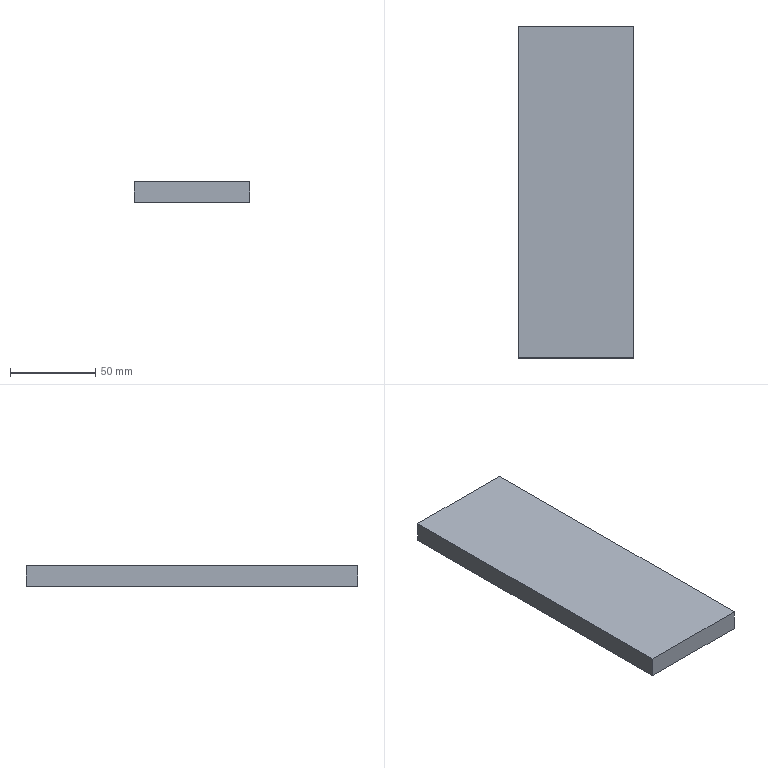Part | SolidWorks | features Extrusion 1 | 1 solid | 6 faces | box 68 x 195 x 12 mm | volume 159120 mm3 | plane 6
STEP:
#1=CARTESIAN_POINT('',(0.,195.,0.));
#2=VERTEX_POINT('',#1);
#3=CARTESIAN_POINT('',(0.,0.,0.));
#4=VERTEX_POINT('',#3);
#5=CARTESIAN_POINT('',(0.,0.,0.));
#6=DIRECTION('',(0.,-1.,0.));
#7=VECTOR('',#6,1000.);
#8=LINE('',#5,#7);
#9=EDGE_CURVE('',#2,#4,#8,.T.);
#10=ORIENTED_EDGE('',*,*,#9,.T.);
#11=CARTESIAN_POINT('',(0.,0.,12.));
#12=VERTEX_POINT('',#11);
#13=CARTESIAN_POINT('',(0.,0.,12.));
#14=DIRECTION('',(0.,0.,-1.));
#15=VECTOR('',#14,1000.);
#16=LINE('',#13,#15);
#17=EDGE_CURVE('',#12,#4,#16,.T.);
#18=ORIENTED_EDGE('',*,*,#17,.F.);
#19=CARTESIAN_POINT('',(0.,195.,12.));
#20=VERTEX_POINT('',#19);
#21=CARTESIAN_POINT('',(0.,0.,12.));
#22=DIRECTION('',(0.,-1.,0.));
#23=VECTOR('',#22,1000.);
#24=LINE('',#21,#23);
#25=EDGE_CURVE('',#20,#12,#24,.T.);
#26=ORIENTED_EDGE('',*,*,#25,.F.);
#27=CARTESIAN_POINT('',(0.,195.,12.));
#28=DIRECTION('',(0.,0.,-1.));
#29=VECTOR('',#28,1000.);
#30=LINE('',#27,#29);
#31=EDGE_CURVE('',#20,#2,#30,.T.);
#32=ORIENTED_EDGE('',*,*,#31,.T.);
#33=EDGE_LOOP('',(#10,#18,#26,#32));
#34=FACE_OUTER_BOUND('',#33,.T.);
#35=CARTESIAN_POINT('',(0.,0.,12.));
#36=DIRECTION('',(1.,0.,0.));
#37=DIRECTION('',(0.,0.,-1.));
#38=AXIS2_PLACEMENT_3D('',#35,#36,#37);
#39=PLANE('',#38);
#40=ADVANCED_FACE('',(#34),#39,.F.);
#41=CARTESIAN_POINT('',(68.,0.,0.));
#42=VERTEX_POINT('',#41);
#43=CARTESIAN_POINT('',(0.,0.,0.));
#44=DIRECTION('',(1.,0.,0.));
#45=VECTOR('',#44,1000.);
#46=LINE('',#43,#45);
#47=EDGE_CURVE('',#4,#42,#46,.T.);
#48=ORIENTED_EDGE('',*,*,#47,.T.);
#49=CARTESIAN_POINT('',(68.,0.,12.));
#50=VERTEX_POINT('',#49);
#51=CARTESIAN_POINT('',(68.,0.,12.));
#52=DIRECTION('',(0.,0.,-1.));
#53=VECTOR('',#52,1000.);
#54=LINE('',#51,#53);
#55=EDGE_CURVE('',#50,#42,#54,.T.);
#56=ORIENTED_EDGE('',*,*,#55,.F.);
#57=CARTESIAN_POINT('',(0.,0.,12.));
#58=DIRECTION('',(1.,0.,0.));
#59=VECTOR('',#58,1000.);
#60=LINE('',#57,#59);
#61=EDGE_CURVE('',#12,#50,#60,.T.);
#62=ORIENTED_EDGE('',*,*,#61,.F.);
#63=ORIENTED_EDGE('',*,*,#17,.T.);
#64=EDGE_LOOP('',(#48,#56,#62,#63));
#65=FACE_OUTER_BOUND('',#64,.T.);
#66=CARTESIAN_POINT('',(0.,0.,12.));
#67=DIRECTION('',(0.,1.,0.));
#68=DIRECTION('',(0.,0.,1.));
#69=AXIS2_PLACEMENT_3D('',#66,#67,#68);
#70=PLANE('',#69);
#71=ADVANCED_FACE('',(#65),#70,.F.);
#72=CARTESIAN_POINT('',(68.,195.,0.));
#73=VERTEX_POINT('',#72);
#74=CARTESIAN_POINT('',(68.,0.,0.));
#75=DIRECTION('',(0.,1.,0.));
#76=VECTOR('',#75,1000.);
#77=LINE('',#74,#76);
#78=EDGE_CURVE('',#42,#73,#77,.T.);
#79=ORIENTED_EDGE('',*,*,#78,.T.);
#80=CARTESIAN_POINT('',(68.,195.,12.));
#81=VERTEX_POINT('',#80);
#82=CARTESIAN_POINT('',(68.,195.,12.));
#83=DIRECTION('',(0.,0.,-1.));
#84=VECTOR('',#83,1000.);
#85=LINE('',#82,#84);
#86=EDGE_CURVE('',#81,#73,#85,.T.);
#87=ORIENTED_EDGE('',*,*,#86,.F.);
#88=CARTESIAN_POINT('',(68.,0.,12.));
#89=DIRECTION('',(0.,1.,0.));
#90=VECTOR('',#89,1000.);
#91=LINE('',#88,#90);
#92=EDGE_CURVE('',#50,#81,#91,.T.);
#93=ORIENTED_EDGE('',*,*,#92,.F.);
#94=ORIENTED_EDGE('',*,*,#55,.T.);
#95=EDGE_LOOP('',(#79,#87,#93,#94));
#96=FACE_OUTER_BOUND('',#95,.T.);
#97=CARTESIAN_POINT('',(68.,0.,12.));
#98=DIRECTION('',(-1.,0.,0.));
#99=DIRECTION('',(0.,0.,1.));
#100=AXIS2_PLACEMENT_3D('',#97,#98,#99);
#101=PLANE('',#100);
#102=ADVANCED_FACE('',(#96),#101,.F.);
#103=CARTESIAN_POINT('',(0.,195.,0.));
#104=DIRECTION('',(-1.,0.,0.));
#105=VECTOR('',#104,1000.);
#106=LINE('',#103,#105);
#107=EDGE_CURVE('',#73,#2,#106,.T.);
#108=ORIENTED_EDGE('',*,*,#107,.T.);
#109=ORIENTED_EDGE('',*,*,#31,.F.);
#110=CARTESIAN_POINT('',(0.,195.,12.));
#111=DIRECTION('',(-1.,0.,0.));
#112=VECTOR('',#111,1000.);
#113=LINE('',#110,#112);
#114=EDGE_CURVE('',#81,#20,#113,.T.);
#115=ORIENTED_EDGE('',*,*,#114,.F.);
#116=ORIENTED_EDGE('',*,*,#86,.T.);
#117=EDGE_LOOP('',(#108,#109,#115,#116));
#118=FACE_OUTER_BOUND('',#117,.T.);
#119=CARTESIAN_POINT('',(0.,195.,12.));
#120=DIRECTION('',(0.,-1.,0.));
#121=DIRECTION('',(0.,0.,-1.));
#122=AXIS2_PLACEMENT_3D('',#119,#120,#121);
#123=PLANE('',#122);
#124=ADVANCED_FACE('',(#118),#123,.F.);
#125=ORIENTED_EDGE('',*,*,#25,.T.);
#126=ORIENTED_EDGE('',*,*,#61,.T.);
#127=ORIENTED_EDGE('',*,*,#92,.T.);
#128=ORIENTED_EDGE('',*,*,#114,.T.);
#129=EDGE_LOOP('',(#125,#126,#127,#128));
#130=FACE_OUTER_BOUND('',#129,.T.);
#131=CARTESIAN_POINT('',(0.,195.,12.));
#132=DIRECTION('',(0.,0.,-1.));
#133=DIRECTION('',(-1.,0.,0.));
#134=AXIS2_PLACEMENT_3D('',#131,#132,#133);
#135=PLANE('',#134);
#136=ADVANCED_FACE('',(#130),#135,.F.);
#137=ORIENTED_EDGE('',*,*,#9,.F.);
#138=ORIENTED_EDGE('',*,*,#107,.F.);
#139=ORIENTED_EDGE('',*,*,#78,.F.);
#140=ORIENTED_EDGE('',*,*,#47,.F.);
#141=EDGE_LOOP('',(#137,#138,#139,#140));
#142=FACE_OUTER_BOUND('',#141,.T.);
#143=CARTESIAN_POINT('',(0.,195.,0.));
#144=DIRECTION('',(0.,0.,-1.));
#145=DIRECTION('',(-1.,0.,0.));
#146=AXIS2_PLACEMENT_3D('',#143,#144,#145);
#147=PLANE('',#146);
#148=ADVANCED_FACE('',(#142),#147,.T.);
#149=CLOSED_SHELL('',(#40,#71,#102,#124,#136,#148));
#150=MANIFOLD_SOLID_BREP('',#149);
#151=CARTESIAN_POINT('',(0.,0.,0.));
#152=DIRECTION('',(0.,0.,1.));
#153=DIRECTION('',(1.,0.,0.));
#154=AXIS2_PLACEMENT_3D('',#151,#152,#153);
#155=(LENGTH_UNIT()NAMED_UNIT(*)SI_UNIT(.MILLI.,.METRE.));
#156=UNCERTAINTY_MEASURE_WITH_UNIT(LENGTH_MEASURE(0.00001),#155,'','');
#157=(NAMED_UNIT(*)PLANE_ANGLE_UNIT()SI_UNIT($,.RADIAN.));
#158=(NAMED_UNIT(*)SI_UNIT($,.STERADIAN.)SOLID_ANGLE_UNIT());
#159=(GEOMETRIC_REPRESENTATION_CONTEXT(3)GLOBAL_UNCERTAINTY_ASSIGNED_CONTEXT((#156))GLOBAL_UNIT_ASSIGNED_CONTEXT((#155,#157,#158))REPRESENTATION_CONTEXT('',''));
#160=ADVANCED_BREP_SHAPE_REPRESENTATION('',(#150,#154),#159);